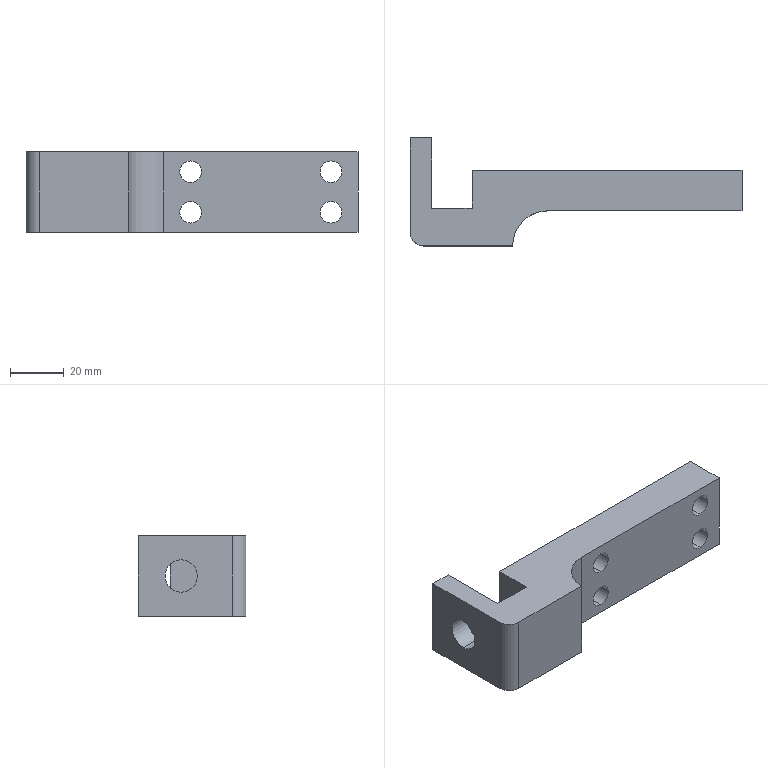Part | SolidWorks | features BaseBody 1 | 1 solid | 23 faces | box 123 x 40 x 30 mm | volume 63756 mm3 | cylinder 12 | plane 11 | commonest cylinder face diameters 8 x8 12 x2 10 x1 26 x1
STEP:
#1=CARTESIAN_POINT('',(340.,-80.,133.121));
#2=VERTEX_POINT('',#1);
#3=CARTESIAN_POINT('',(340.,-80.,141.121));
#4=VERTEX_POINT('',#3);
#5=CARTESIAN_POINT('',(340.,-80.,137.121));
#6=DIRECTION('',(0.,1.,0.));
#7=DIRECTION('',(0.,0.,-1.));
#8=AXIS2_PLACEMENT_3D('',#5,#6,#7);
#9=CIRCLE('',#8,4.);
#10=EDGE_CURVE('',#2,#4,#9,.T.);
#11=ORIENTED_EDGE('',*,*,#10,.T.);
#12=CARTESIAN_POINT('',(340.,-95.,141.121));
#13=VERTEX_POINT('',#12);
#14=CARTESIAN_POINT('',(340.,-95.,141.121));
#15=DIRECTION('',(0.,-1.,0.));
#16=VECTOR('',#15,1000.);
#17=LINE('',#14,#16);
#18=EDGE_CURVE('',#4,#13,#17,.T.);
#19=ORIENTED_EDGE('',*,*,#18,.T.);
#20=CARTESIAN_POINT('',(340.,-95.,133.121));
#21=VERTEX_POINT('',#20);
#22=CARTESIAN_POINT('',(340.,-95.,137.121));
#23=DIRECTION('',(0.,1.,0.));
#24=DIRECTION('',(0.,0.,-1.));
#25=AXIS2_PLACEMENT_3D('',#22,#23,#24);
#26=CIRCLE('',#25,4.);
#27=EDGE_CURVE('',#21,#13,#26,.T.);
#28=ORIENTED_EDGE('',*,*,#27,.F.);
#29=CARTESIAN_POINT('',(340.,-95.,133.121));
#30=DIRECTION('',(0.,-1.,0.));
#31=VECTOR('',#30,1000.);
#32=LINE('',#29,#31);
#33=EDGE_CURVE('',#2,#21,#32,.T.);
#34=ORIENTED_EDGE('',*,*,#33,.F.);
#35=EDGE_LOOP('',(#11,#19,#28,#34));
#36=FACE_OUTER_BOUND('',#35,.T.);
#37=CARTESIAN_POINT('',(340.,-95.,137.121));
#38=DIRECTION('',(0.,-1.,0.));
#39=DIRECTION('',(0.,0.,-1.));
#40=AXIS2_PLACEMENT_3D('',#37,#38,#39);
#41=CYLINDRICAL_SURFACE('',#40,4.);
#42=ADVANCED_FACE('',(#36),#41,.F.);
#43=CARTESIAN_POINT('',(340.,-80.,148.121));
#44=VERTEX_POINT('',#43);
#45=CARTESIAN_POINT('',(340.,-80.,156.121));
#46=VERTEX_POINT('',#45);
#47=CARTESIAN_POINT('',(340.,-80.,152.121));
#48=DIRECTION('',(0.,1.,0.));
#49=DIRECTION('',(0.,0.,-1.));
#50=AXIS2_PLACEMENT_3D('',#47,#48,#49);
#51=CIRCLE('',#50,4.);
#52=EDGE_CURVE('',#44,#46,#51,.T.);
#53=ORIENTED_EDGE('',*,*,#52,.T.);
#54=CARTESIAN_POINT('',(340.,-95.,156.121));
#55=VERTEX_POINT('',#54);
#56=CARTESIAN_POINT('',(340.,-95.,156.121));
#57=DIRECTION('',(0.,-1.,0.));
#58=VECTOR('',#57,1000.);
#59=LINE('',#56,#58);
#60=EDGE_CURVE('',#46,#55,#59,.T.);
#61=ORIENTED_EDGE('',*,*,#60,.T.);
#62=CARTESIAN_POINT('',(340.,-95.,148.121));
#63=VERTEX_POINT('',#62);
#64=CARTESIAN_POINT('',(340.,-95.,152.121));
#65=DIRECTION('',(0.,1.,0.));
#66=DIRECTION('',(0.,0.,-1.));
#67=AXIS2_PLACEMENT_3D('',#64,#65,#66);
#68=CIRCLE('',#67,4.);
#69=EDGE_CURVE('',#63,#55,#68,.T.);
#70=ORIENTED_EDGE('',*,*,#69,.F.);
#71=CARTESIAN_POINT('',(340.,-95.,148.121));
#72=DIRECTION('',(0.,-1.,0.));
#73=VECTOR('',#72,1000.);
#74=LINE('',#71,#73);
#75=EDGE_CURVE('',#44,#63,#74,.T.);
#76=ORIENTED_EDGE('',*,*,#75,.F.);
#77=EDGE_LOOP('',(#53,#61,#70,#76));
#78=FACE_OUTER_BOUND('',#77,.T.);
#79=CARTESIAN_POINT('',(340.,-95.,152.121));
#80=DIRECTION('',(0.,-1.,0.));
#81=DIRECTION('',(0.,0.,-1.));
#82=AXIS2_PLACEMENT_3D('',#79,#80,#81);
#83=CYLINDRICAL_SURFACE('',#82,4.);
#84=ADVANCED_FACE('',(#78),#83,.F.);
#85=CARTESIAN_POINT('',(288.,-80.,148.121));
#86=VERTEX_POINT('',#85);
#87=CARTESIAN_POINT('',(288.,-80.,156.121));
#88=VERTEX_POINT('',#87);
#89=CARTESIAN_POINT('',(288.,-80.,152.121));
#90=DIRECTION('',(0.,1.,0.));
#91=DIRECTION('',(0.,0.,-1.));
#92=AXIS2_PLACEMENT_3D('',#89,#90,#91);
#93=CIRCLE('',#92,4.);
#94=EDGE_CURVE('',#86,#88,#93,.T.);
#95=ORIENTED_EDGE('',*,*,#94,.T.);
#96=CARTESIAN_POINT('',(288.,-95.,156.121));
#97=VERTEX_POINT('',#96);
#98=CARTESIAN_POINT('',(288.,-95.,156.121));
#99=DIRECTION('',(0.,-1.,0.));
#100=VECTOR('',#99,1000.);
#101=LINE('',#98,#100);
#102=EDGE_CURVE('',#88,#97,#101,.T.);
#103=ORIENTED_EDGE('',*,*,#102,.T.);
#104=CARTESIAN_POINT('',(288.,-95.,148.121));
#105=VERTEX_POINT('',#104);
#106=CARTESIAN_POINT('',(288.,-95.,152.121));
#107=DIRECTION('',(0.,1.,0.));
#108=DIRECTION('',(0.,0.,-1.));
#109=AXIS2_PLACEMENT_3D('',#106,#107,#108);
#110=CIRCLE('',#109,4.);
#111=EDGE_CURVE('',#105,#97,#110,.T.);
#112=ORIENTED_EDGE('',*,*,#111,.F.);
#113=CARTESIAN_POINT('',(288.,-95.,148.121));
#114=DIRECTION('',(0.,-1.,0.));
#115=VECTOR('',#114,1000.);
#116=LINE('',#113,#115);
#117=EDGE_CURVE('',#86,#105,#116,.T.);
#118=ORIENTED_EDGE('',*,*,#117,.F.);
#119=EDGE_LOOP('',(#95,#103,#112,#118));
#120=FACE_OUTER_BOUND('',#119,.T.);
#121=CARTESIAN_POINT('',(288.,-95.,152.121));
#122=DIRECTION('',(0.,-1.,0.));
#123=DIRECTION('',(0.,0.,-1.));
#124=AXIS2_PLACEMENT_3D('',#121,#122,#123);
#125=CYLINDRICAL_SURFACE('',#124,4.);
#126=ADVANCED_FACE('',(#120),#125,.F.);
#127=CARTESIAN_POINT('',(288.,-80.,133.121));
#128=VERTEX_POINT('',#127);
#129=CARTESIAN_POINT('',(288.,-80.,141.121));
#130=VERTEX_POINT('',#129);
#131=CARTESIAN_POINT('',(288.,-80.,137.121));
#132=DIRECTION('',(0.,1.,0.));
#133=DIRECTION('',(0.,0.,-1.));
#134=AXIS2_PLACEMENT_3D('',#131,#132,#133);
#135=CIRCLE('',#134,4.);
#136=EDGE_CURVE('',#128,#130,#135,.T.);
#137=ORIENTED_EDGE('',*,*,#136,.T.);
#138=CARTESIAN_POINT('',(288.,-95.,141.121));
#139=VERTEX_POINT('',#138);
#140=CARTESIAN_POINT('',(288.,-95.,141.121));
#141=DIRECTION('',(0.,-1.,0.));
#142=VECTOR('',#141,1000.);
#143=LINE('',#140,#142);
#144=EDGE_CURVE('',#130,#139,#143,.T.);
#145=ORIENTED_EDGE('',*,*,#144,.T.);
#146=CARTESIAN_POINT('',(288.,-95.,133.121));
#147=VERTEX_POINT('',#146);
#148=CARTESIAN_POINT('',(288.,-95.,137.121));
#149=DIRECTION('',(0.,1.,0.));
#150=DIRECTION('',(0.,0.,-1.));
#151=AXIS2_PLACEMENT_3D('',#148,#149,#150);
#152=CIRCLE('',#151,4.);
#153=EDGE_CURVE('',#147,#139,#152,.T.);
#154=ORIENTED_EDGE('',*,*,#153,.F.);
#155=CARTESIAN_POINT('',(288.,-95.,133.121));
#156=DIRECTION('',(0.,-1.,0.));
#157=VECTOR('',#156,1000.);
#158=LINE('',#155,#157);
#159=EDGE_CURVE('',#128,#147,#158,.T.);
#160=ORIENTED_EDGE('',*,*,#159,.F.);
#161=EDGE_LOOP('',(#137,#145,#154,#160));
#162=FACE_OUTER_BOUND('',#161,.T.);
#163=CARTESIAN_POINT('',(288.,-95.,137.121));
#164=DIRECTION('',(0.,-1.,0.));
#165=DIRECTION('',(0.,0.,-1.));
#166=AXIS2_PLACEMENT_3D('',#163,#164,#165);
#167=CYLINDRICAL_SURFACE('',#166,4.);
#168=ADVANCED_FACE('',(#162),#167,.F.);
#169=CARTESIAN_POINT('',(235.,-84.,150.621));
#170=VERTEX_POINT('',#169);
#171=CARTESIAN_POINT('',(235.,-84.,138.621));
#172=VERTEX_POINT('',#171);
#173=CARTESIAN_POINT('',(235.,-84.,144.621));
#174=DIRECTION('',(1.,0.,0.));
#175=DIRECTION('',(0.,0.,1.));
#176=AXIS2_PLACEMENT_3D('',#173,#174,#175);
#177=CIRCLE('',#176,6.);
#178=EDGE_CURVE('',#170,#172,#177,.T.);
#179=ORIENTED_EDGE('',*,*,#178,.T.);
#180=CARTESIAN_POINT('',(227.,-84.,138.621));
#181=VERTEX_POINT('',#180);
#182=CARTESIAN_POINT('',(251.971,-84.,138.621));
#183=DIRECTION('',(-1.,0.,0.));
#184=VECTOR('',#183,1000.);
#185=LINE('',#182,#184);
#186=EDGE_CURVE('',#172,#181,#185,.T.);
#187=ORIENTED_EDGE('',*,*,#186,.T.);
#188=CARTESIAN_POINT('',(227.,-84.,150.621));
#189=VERTEX_POINT('',#188);
#190=CARTESIAN_POINT('',(227.,-84.,144.621));
#191=DIRECTION('',(-1.,0.,0.));
#192=DIRECTION('',(0.,0.,1.));
#193=AXIS2_PLACEMENT_3D('',#190,#191,#192);
#194=CIRCLE('',#193,6.);
#195=EDGE_CURVE('',#181,#189,#194,.T.);
#196=ORIENTED_EDGE('',*,*,#195,.T.);
#197=CARTESIAN_POINT('',(251.971,-84.,150.621));
#198=DIRECTION('',(-1.,0.,0.));
#199=VECTOR('',#198,1000.);
#200=LINE('',#197,#199);
#201=EDGE_CURVE('',#170,#189,#200,.T.);
#202=ORIENTED_EDGE('',*,*,#201,.F.);
#203=EDGE_LOOP('',(#179,#187,#196,#202));
#204=FACE_OUTER_BOUND('',#203,.T.);
#205=CARTESIAN_POINT('',(251.971,-84.,144.621));
#206=DIRECTION('',(-1.,0.,0.));
#207=DIRECTION('',(0.,0.,1.));
#208=AXIS2_PLACEMENT_3D('',#205,#206,#207);
#209=CYLINDRICAL_SURFACE('',#208,6.);
#210=ADVANCED_FACE('',(#204),#209,.F.);
#211=CARTESIAN_POINT('',(350.,-80.,129.621));
#212=VERTEX_POINT('',#211);
#213=CARTESIAN_POINT('',(350.,-80.,159.621));
#214=VERTEX_POINT('',#213);
#215=CARTESIAN_POINT('',(350.,-80.,129.621));
#216=DIRECTION('',(0.,0.,1.));
#217=VECTOR('',#216,1000.);
#218=LINE('',#215,#217);
#219=EDGE_CURVE('',#212,#214,#218,.T.);
#220=ORIENTED_EDGE('',*,*,#219,.F.);
#221=CARTESIAN_POINT('',(250.,-80.,129.621));
#222=VERTEX_POINT('',#221);
#223=CARTESIAN_POINT('',(350.,-80.,129.621));
#224=DIRECTION('',(1.,0.,0.));
#225=VECTOR('',#224,1000.);
#226=LINE('',#223,#225);
#227=EDGE_CURVE('',#222,#212,#226,.T.);
#228=ORIENTED_EDGE('',*,*,#227,.F.);
#229=CARTESIAN_POINT('',(250.,-80.,159.621));
#230=VERTEX_POINT('',#229);
#231=CARTESIAN_POINT('',(250.,-80.,129.621));
#232=DIRECTION('',(0.,0.,-1.));
#233=VECTOR('',#232,1000.);
#234=LINE('',#231,#233);
#235=EDGE_CURVE('',#230,#222,#234,.T.);
#236=ORIENTED_EDGE('',*,*,#235,.F.);
#237=CARTESIAN_POINT('',(350.,-80.,159.621));
#238=DIRECTION('',(-1.,0.,0.));
#239=VECTOR('',#238,1000.);
#240=LINE('',#237,#239);
#241=EDGE_CURVE('',#214,#230,#240,.T.);
#242=ORIENTED_EDGE('',*,*,#241,.F.);
#243=EDGE_LOOP('',(#220,#228,#236,#242));
#244=FACE_OUTER_BOUND('',#243,.T.);
#245=ORIENTED_EDGE('',*,*,#10,.F.);
#246=CARTESIAN_POINT('',(340.,-80.,137.121));
#247=DIRECTION('',(0.,1.,0.));
#248=DIRECTION('',(0.,0.,-1.));
#249=AXIS2_PLACEMENT_3D('',#246,#247,#248);
#250=CIRCLE('',#249,4.);
#251=EDGE_CURVE('',#4,#2,#250,.T.);
#252=ORIENTED_EDGE('',*,*,#251,.F.);
#253=EDGE_LOOP('',(#245,#252));
#254=FACE_BOUND('',#253,.T.);
#255=ORIENTED_EDGE('',*,*,#52,.F.);
#256=CARTESIAN_POINT('',(340.,-80.,152.121));
#257=DIRECTION('',(0.,1.,0.));
#258=DIRECTION('',(0.,0.,-1.));
#259=AXIS2_PLACEMENT_3D('',#256,#257,#258);
#260=CIRCLE('',#259,4.);
#261=EDGE_CURVE('',#46,#44,#260,.T.);
#262=ORIENTED_EDGE('',*,*,#261,.F.);
#263=EDGE_LOOP('',(#255,#262));
#264=FACE_BOUND('',#263,.T.);
#265=ORIENTED_EDGE('',*,*,#94,.F.);
#266=CARTESIAN_POINT('',(288.,-80.,152.121));
#267=DIRECTION('',(0.,1.,0.));
#268=DIRECTION('',(0.,0.,-1.));
#269=AXIS2_PLACEMENT_3D('',#266,#267,#268);
#270=CIRCLE('',#269,4.);
#271=EDGE_CURVE('',#88,#86,#270,.T.);
#272=ORIENTED_EDGE('',*,*,#271,.F.);
#273=EDGE_LOOP('',(#265,#272));
#274=FACE_BOUND('',#273,.T.);
#275=ORIENTED_EDGE('',*,*,#136,.F.);
#276=CARTESIAN_POINT('',(288.,-80.,137.121));
#277=DIRECTION('',(0.,1.,0.));
#278=DIRECTION('',(0.,0.,-1.));
#279=AXIS2_PLACEMENT_3D('',#276,#277,#278);
#280=CIRCLE('',#279,4.);
#281=EDGE_CURVE('',#130,#128,#280,.T.);
#282=ORIENTED_EDGE('',*,*,#281,.F.);
#283=EDGE_LOOP('',(#275,#282));
#284=FACE_BOUND('',#283,.T.);
#285=CARTESIAN_POINT('',(350.,-80.,129.621));
#286=DIRECTION('',(0.,-1.,0.));
#287=DIRECTION('',(0.,0.,-1.));
#288=AXIS2_PLACEMENT_3D('',#285,#286,#287);
#289=PLANE('',#288);
#290=ADVANCED_FACE('',(#244,#254,#264,#274,#284),#289,.F.);
#291=CARTESIAN_POINT('',(232.,-108.,159.621));
#292=VERTEX_POINT('',#291);
#293=CARTESIAN_POINT('',(227.,-103.,159.621));
#294=VERTEX_POINT('',#293);
#295=CARTESIAN_POINT('',(232.,-103.,159.621));
#296=DIRECTION('',(0.,0.,-1.));
#297=DIRECTION('',(1.,0.,0.));
#298=AXIS2_PLACEMENT_3D('',#295,#296,#297);
#299=CIRCLE('',#298,5.);
#300=EDGE_CURVE('',#292,#294,#299,.T.);
#301=ORIENTED_EDGE('',*,*,#300,.F.);
#302=CARTESIAN_POINT('',(265.,-108.,159.621));
#303=VERTEX_POINT('',#302);
#304=CARTESIAN_POINT('',(251.867,-108.,159.621));
#305=DIRECTION('',(-1.,0.,0.));
#306=VECTOR('',#305,1000.);
#307=LINE('',#304,#306);
#308=EDGE_CURVE('',#303,#292,#307,.T.);
#309=ORIENTED_EDGE('',*,*,#308,.F.);
#310=CARTESIAN_POINT('',(278.,-95.,159.621));
#311=VERTEX_POINT('',#310);
#312=CARTESIAN_POINT('',(278.,-108.,159.621));
#313=DIRECTION('',(0.,0.,1.));
#314=DIRECTION('',(-1.,0.,0.));
#315=AXIS2_PLACEMENT_3D('',#312,#313,#314);
#316=CIRCLE('',#315,13.);
#317=EDGE_CURVE('',#311,#303,#316,.T.);
#318=ORIENTED_EDGE('',*,*,#317,.F.);
#319=CARTESIAN_POINT('',(350.,-95.,159.621));
#320=VERTEX_POINT('',#319);
#321=CARTESIAN_POINT('',(251.867,-95.,159.621));
#322=DIRECTION('',(-1.,0.,0.));
#323=VECTOR('',#322,1000.);
#324=LINE('',#321,#323);
#325=EDGE_CURVE('',#320,#311,#324,.T.);
#326=ORIENTED_EDGE('',*,*,#325,.F.);
#327=CARTESIAN_POINT('',(350.,-82.6,159.621));
#328=DIRECTION('',(0.,-1.,0.));
#329=VECTOR('',#328,1000.);
#330=LINE('',#327,#329);
#331=EDGE_CURVE('',#214,#320,#330,.T.);
#332=ORIENTED_EDGE('',*,*,#331,.F.);
#333=ORIENTED_EDGE('',*,*,#241,.T.);
#334=CARTESIAN_POINT('',(250.,-94.,159.621));
#335=VERTEX_POINT('',#334);
#336=CARTESIAN_POINT('',(250.,-82.6,159.621));
#337=DIRECTION('',(0.,1.,0.));
#338=VECTOR('',#337,1000.);
#339=LINE('',#336,#338);
#340=EDGE_CURVE('',#335,#230,#339,.T.);
#341=ORIENTED_EDGE('',*,*,#340,.F.);
#342=CARTESIAN_POINT('',(235.,-94.,159.621));
#343=VERTEX_POINT('',#342);
#344=CARTESIAN_POINT('',(251.867,-94.,159.621));
#345=DIRECTION('',(1.,0.,0.));
#346=VECTOR('',#345,1000.);
#347=LINE('',#344,#346);
#348=EDGE_CURVE('',#343,#335,#347,.T.);
#349=ORIENTED_EDGE('',*,*,#348,.F.);
#350=CARTESIAN_POINT('',(235.,-68.,159.621));
#351=VERTEX_POINT('',#350);
#352=CARTESIAN_POINT('',(235.,-82.6,159.621));
#353=DIRECTION('',(0.,-1.,0.));
#354=VECTOR('',#353,1000.);
#355=LINE('',#352,#354);
#356=EDGE_CURVE('',#351,#343,#355,.T.);
#357=ORIENTED_EDGE('',*,*,#356,.F.);
#358=CARTESIAN_POINT('',(227.,-68.,159.621));
#359=VERTEX_POINT('',#358);
#360=CARTESIAN_POINT('',(251.867,-68.,159.621));
#361=DIRECTION('',(1.,0.,0.));
#362=VECTOR('',#361,1000.);
#363=LINE('',#360,#362);
#364=EDGE_CURVE('',#359,#351,#363,.T.);
#365=ORIENTED_EDGE('',*,*,#364,.F.);
#366=CARTESIAN_POINT('',(227.,-82.6,159.621));
#367=DIRECTION('',(0.,1.,0.));
#368=VECTOR('',#367,1000.);
#369=LINE('',#366,#368);
#370=EDGE_CURVE('',#294,#359,#369,.T.);
#371=ORIENTED_EDGE('',*,*,#370,.F.);
#372=EDGE_LOOP('',(#301,#309,#318,#326,#332,#333,#341,#349,#357,#365,#371));
#373=FACE_OUTER_BOUND('',#372,.T.);
#374=CARTESIAN_POINT('',(251.867,-82.6,159.621));
#375=DIRECTION('',(0.,0.,-1.));
#376=DIRECTION('',(-1.,0.,0.));
#377=AXIS2_PLACEMENT_3D('',#374,#375,#376);
#378=PLANE('',#377);
#379=ADVANCED_FACE('',(#373),#378,.F.);
#380=CARTESIAN_POINT('',(350.,-95.,129.621));
#381=VERTEX_POINT('',#380);
#382=CARTESIAN_POINT('',(350.,-95.,129.621));
#383=DIRECTION('',(0.,0.,1.));
#384=VECTOR('',#383,1000.);
#385=LINE('',#382,#384);
#386=EDGE_CURVE('',#381,#320,#385,.T.);
#387=ORIENTED_EDGE('',*,*,#386,.F.);
#388=CARTESIAN_POINT('',(350.,-80.,129.621));
#389=DIRECTION('',(0.,-1.,0.));
#390=VECTOR('',#389,1000.);
#391=LINE('',#388,#390);
#392=EDGE_CURVE('',#212,#381,#391,.T.);
#393=ORIENTED_EDGE('',*,*,#392,.F.);
#394=ORIENTED_EDGE('',*,*,#219,.T.);
#395=ORIENTED_EDGE('',*,*,#331,.T.);
#396=EDGE_LOOP('',(#387,#393,#394,#395));
#397=FACE_OUTER_BOUND('',#396,.T.);
#398=CARTESIAN_POINT('',(350.,-80.,129.621));
#399=DIRECTION('',(-1.,0.,0.));
#400=DIRECTION('',(0.,0.,1.));
#401=AXIS2_PLACEMENT_3D('',#398,#399,#400);
#402=PLANE('',#401);
#403=ADVANCED_FACE('',(#397),#402,.F.);
#404=CARTESIAN_POINT('',(278.,-95.,129.621));
#405=VERTEX_POINT('',#404);
#406=CARTESIAN_POINT('',(251.867,-95.,129.621));
#407=DIRECTION('',(-1.,0.,0.));
#408=VECTOR('',#407,1000.);
#409=LINE('',#406,#408);
#410=EDGE_CURVE('',#381,#405,#409,.T.);
#411=ORIENTED_EDGE('',*,*,#410,.T.);
#412=CARTESIAN_POINT('',(265.,-108.,129.621));
#413=VERTEX_POINT('',#412);
#414=CARTESIAN_POINT('',(278.,-108.,129.621));
#415=DIRECTION('',(0.,0.,1.));
#416=DIRECTION('',(-1.,0.,0.));
#417=AXIS2_PLACEMENT_3D('',#414,#415,#416);
#418=CIRCLE('',#417,13.);
#419=EDGE_CURVE('',#405,#413,#418,.T.);
#420=ORIENTED_EDGE('',*,*,#419,.T.);
#421=CARTESIAN_POINT('',(232.,-108.,129.621));
#422=VERTEX_POINT('',#421);
#423=CARTESIAN_POINT('',(251.867,-108.,129.621));
#424=DIRECTION('',(-1.,0.,0.));
#425=VECTOR('',#424,1000.);
#426=LINE('',#423,#425);
#427=EDGE_CURVE('',#413,#422,#426,.T.);
#428=ORIENTED_EDGE('',*,*,#427,.T.);
#429=CARTESIAN_POINT('',(227.,-103.,129.621));
#430=VERTEX_POINT('',#429);
#431=CARTESIAN_POINT('',(232.,-103.,129.621));
#432=DIRECTION('',(0.,0.,-1.));
#433=DIRECTION('',(1.,0.,0.));
#434=AXIS2_PLACEMENT_3D('',#431,#432,#433);
#435=CIRCLE('',#434,5.);
#436=EDGE_CURVE('',#422,#430,#435,.T.);
#437=ORIENTED_EDGE('',*,*,#436,.T.);
#438=CARTESIAN_POINT('',(227.,-68.,129.621));
#439=VERTEX_POINT('',#438);
#440=CARTESIAN_POINT('',(227.,-82.6,129.621));
#441=DIRECTION('',(0.,1.,0.));
#442=VECTOR('',#441,1000.);
#443=LINE('',#440,#442);
#444=EDGE_CURVE('',#430,#439,#443,.T.);
#445=ORIENTED_EDGE('',*,*,#444,.T.);
#446=CARTESIAN_POINT('',(235.,-68.,129.621));
#447=VERTEX_POINT('',#446);
#448=CARTESIAN_POINT('',(251.867,-68.,129.621));
#449=DIRECTION('',(1.,0.,0.));
#450=VECTOR('',#449,1000.);
#451=LINE('',#448,#450);
#452=EDGE_CURVE('',#439,#447,#451,.T.);
#453=ORIENTED_EDGE('',*,*,#452,.T.);
#454=CARTESIAN_POINT('',(235.,-94.,129.621));
#455=VERTEX_POINT('',#454);
#456=CARTESIAN_POINT('',(235.,-82.6,129.621));
#457=DIRECTION('',(0.,-1.,0.));
#458=VECTOR('',#457,1000.);
#459=LINE('',#456,#458);
#460=EDGE_CURVE('',#447,#455,#459,.T.);
#461=ORIENTED_EDGE('',*,*,#460,.T.);
#462=CARTESIAN_POINT('',(250.,-94.,129.621));
#463=VERTEX_POINT('',#462);
#464=CARTESIAN_POINT('',(251.867,-94.,129.621));
#465=DIRECTION('',(1.,0.,0.));
#466=VECTOR('',#465,1000.);
#467=LINE('',#464,#466);
#468=EDGE_CURVE('',#455,#463,#467,.T.);
#469=ORIENTED_EDGE('',*,*,#468,.T.);
#470=CARTESIAN_POINT('',(250.,-82.6,129.621));
#471=DIRECTION('',(0.,1.,0.));
#472=VECTOR('',#471,1000.);
#473=LINE('',#470,#472);
#474=EDGE_CURVE('',#463,#222,#473,.T.);
#475=ORIENTED_EDGE('',*,*,#474,.T.);
#476=ORIENTED_EDGE('',*,*,#227,.T.);
#477=ORIENTED_EDGE('',*,*,#392,.T.);
#478=EDGE_LOOP('',(#411,#420,#428,#437,#445,#453,#461,#469,#475,#476,#477));
#479=FACE_OUTER_BOUND('',#478,.T.);
#480=CARTESIAN_POINT('',(251.867,-82.6,129.621));
#481=DIRECTION('',(0.,0.,-1.));
#482=DIRECTION('',(-1.,0.,0.));
#483=AXIS2_PLACEMENT_3D('',#480,#481,#482);
#484=PLANE('',#483);
#485=ADVANCED_FACE('',(#479),#484,.T.);
#486=ORIENTED_EDGE('',*,*,#235,.T.);
#487=ORIENTED_EDGE('',*,*,#474,.F.);
#488=CARTESIAN_POINT('',(250.,-94.,129.621));
#489=DIRECTION('',(0.,0.,-1.));
#490=VECTOR('',#489,1000.);
#491=LINE('',#488,#490);
#492=EDGE_CURVE('',#335,#463,#491,.T.);
#493=ORIENTED_EDGE('',*,*,#492,.F.);
#494=ORIENTED_EDGE('',*,*,#340,.T.);
#495=EDGE_LOOP('',(#486,#487,#493,#494));
#496=FACE_OUTER_BOUND('',#495,.T.);
#497=CARTESIAN_POINT('',(250.,-80.,129.621));
#498=DIRECTION('',(1.,0.,0.));
#499=DIRECTION('',(0.,0.,-1.));
#500=AXIS2_PLACEMENT_3D('',#497,#498,#499);
#501=PLANE('',#500);
#502=ADVANCED_FACE('',(#496),#501,.F.);
#503=ORIENTED_EDGE('',*,*,#18,.F.);
#504=ORIENTED_EDGE('',*,*,#251,.T.);
#505=ORIENTED_EDGE('',*,*,#33,.T.);
#506=CARTESIAN_POINT('',(340.,-95.,137.121));
#507=DIRECTION('',(0.,1.,0.));
#508=DIRECTION('',(0.,0.,-1.));
#509=AXIS2_PLACEMENT_3D('',#506,#507,#508);
#510=CIRCLE('',#509,4.);
#511=EDGE_CURVE('',#13,#21,#510,.T.);
#512=ORIENTED_EDGE('',*,*,#511,.F.);
#513=EDGE_LOOP('',(#503,#504,#505,#512));
#514=FACE_OUTER_BOUND('',#513,.T.);
#515=CARTESIAN_POINT('',(340.,-95.,137.121));
#516=DIRECTION('',(0.,-1.,0.));
#517=DIRECTION('',(0.,0.,-1.));
#518=AXIS2_PLACEMENT_3D('',#515,#516,#517);
#519=CYLINDRICAL_SURFACE('',#518,4.);
#520=ADVANCED_FACE('',(#514),#519,.F.);
#521=ORIENTED_EDGE('',*,*,#60,.F.);
#522=ORIENTED_EDGE('',*,*,#261,.T.);
#523=ORIENTED_EDGE('',*,*,#75,.T.);
#524=CARTESIAN_POINT('',(340.,-95.,152.121));
#525=DIRECTION('',(0.,1.,0.));
#526=DIRECTION('',(0.,0.,-1.));
#527=AXIS2_PLACEMENT_3D('',#524,#525,#526);
#528=CIRCLE('',#527,4.);
#529=EDGE_CURVE('',#55,#63,#528,.T.);
#530=ORIENTED_EDGE('',*,*,#529,.F.);
#531=EDGE_LOOP('',(#521,#522,#523,#530));
#532=FACE_OUTER_BOUND('',#531,.T.);
#533=CARTESIAN_POINT('',(340.,-95.,152.121));
#534=DIRECTION('',(0.,-1.,0.));
#535=DIRECTION('',(0.,0.,-1.));
#536=AXIS2_PLACEMENT_3D('',#533,#534,#535);
#537=CYLINDRICAL_SURFACE('',#536,4.);
#538=ADVANCED_FACE('',(#532),#537,.F.);
#539=ORIENTED_EDGE('',*,*,#102,.F.);
#540=ORIENTED_EDGE('',*,*,#271,.T.);
#541=ORIENTED_EDGE('',*,*,#117,.T.);
#542=CARTESIAN_POINT('',(288.,-95.,152.121));
#543=DIRECTION('',(0.,1.,0.));
#544=DIRECTION('',(0.,0.,-1.));
#545=AXIS2_PLACEMENT_3D('',#542,#543,#544);
#546=CIRCLE('',#545,4.);
#547=EDGE_CURVE('',#97,#105,#546,.T.);
#548=ORIENTED_EDGE('',*,*,#547,.F.);
#549=EDGE_LOOP('',(#539,#540,#541,#548));
#550=FACE_OUTER_BOUND('',#549,.T.);
#551=CARTESIAN_POINT('',(288.,-95.,152.121));
#552=DIRECTION('',(0.,-1.,0.));
#553=DIRECTION('',(0.,0.,-1.));
#554=AXIS2_PLACEMENT_3D('',#551,#552,#553);
#555=CYLINDRICAL_SURFACE('',#554,4.);
#556=ADVANCED_FACE('',(#550),#555,.F.);
#557=ORIENTED_EDGE('',*,*,#144,.F.);
#558=ORIENTED_EDGE('',*,*,#281,.T.);
#559=ORIENTED_EDGE('',*,*,#159,.T.);
#560=CARTESIAN_POINT('',(288.,-95.,137.121));
#561=DIRECTION('',(0.,1.,0.));
#562=DIRECTION('',(0.,0.,-1.));
#563=AXIS2_PLACEMENT_3D('',#560,#561,#562);
#564=CIRCLE('',#563,4.);
#565=EDGE_CURVE('',#139,#147,#564,.T.);
#566=ORIENTED_EDGE('',*,*,#565,.F.);
#567=EDGE_LOOP('',(#557,#558,#559,#566));
#568=FACE_OUTER_BOUND('',#567,.T.);
#569=CARTESIAN_POINT('',(288.,-95.,137.121));
#570=DIRECTION('',(0.,-1.,0.));
#571=DIRECTION('',(0.,0.,-1.));
#572=AXIS2_PLACEMENT_3D('',#569,#570,#571);
#573=CYLINDRICAL_SURFACE('',#572,4.);
#574=ADVANCED_FACE('',(#568),#573,.F.);
#575=CARTESIAN_POINT('',(227.,-103.,129.621));
#576=DIRECTION('',(0.,0.,-1.));
#577=VECTOR('',#576,1000.);
#578=LINE('',#575,#577);
#579=EDGE_CURVE('',#294,#430,#578,.T.);
#580=ORIENTED_EDGE('',*,*,#579,.F.);
#581=ORIENTED_EDGE('',*,*,#370,.T.);
#582=CARTESIAN_POINT('',(227.,-68.,129.621));
#583=DIRECTION('',(0.,0.,1.));
#584=VECTOR('',#583,1000.);
#585=LINE('',#582,#584);
#586=EDGE_CURVE('',#439,#359,#585,.T.);
#587=ORIENTED_EDGE('',*,*,#586,.F.);
#588=ORIENTED_EDGE('',*,*,#444,.F.);
#589=EDGE_LOOP('',(#580,#581,#587,#588));
#590=FACE_OUTER_BOUND('',#589,.T.);
#591=CARTESIAN_POINT('',(227.,-84.,144.621));
#592=DIRECTION('',(-1.,0.,0.));
#593=DIRECTION('',(0.,0.,1.));
#594=AXIS2_PLACEMENT_3D('',#591,#592,#593);
#595=CIRCLE('',#594,6.);
#596=EDGE_CURVE('',#189,#181,#595,.T.);
#597=ORIENTED_EDGE('',*,*,#596,.F.);
#598=ORIENTED_EDGE('',*,*,#195,.F.);
#599=EDGE_LOOP('',(#597,#598));
#600=FACE_BOUND('',#599,.T.);
#601=CARTESIAN_POINT('',(227.,-93.,129.621));
#602=DIRECTION('',(1.,0.,0.));
#603=DIRECTION('',(0.,0.,-1.));
#604=AXIS2_PLACEMENT_3D('',#601,#602,#603);
#605=PLANE('',#604);
#606=ADVANCED_FACE('',(#590,#600),#605,.F.);
#607=ORIENTED_EDGE('',*,*,#300,.T.);
#608=ORIENTED_EDGE('',*,*,#579,.T.);
#609=ORIENTED_EDGE('',*,*,#436,.F.);
#610=CARTESIAN_POINT('',(232.,-108.,129.621));
#611=DIRECTION('',(0.,0.,1.));
#612=VECTOR('',#611,1000.);
#613=LINE('',#610,#612);
#614=EDGE_CURVE('',#422,#292,#613,.T.);
#615=ORIENTED_EDGE('',*,*,#614,.T.);
#616=EDGE_LOOP('',(#607,#608,#609,#615));
#617=FACE_OUTER_BOUND('',#616,.T.);
#618=CARTESIAN_POINT('',(232.,-103.,129.621));
#619=DIRECTION('',(0.,0.,1.));
#620=DIRECTION('',(1.,0.,0.));
#621=AXIS2_PLACEMENT_3D('',#618,#619,#620);
#622=CYLINDRICAL_SURFACE('',#621,5.);
#623=ADVANCED_FACE('',(#617),#622,.T.);
#624=ORIENTED_EDGE('',*,*,#614,.F.);
#625=ORIENTED_EDGE('',*,*,#427,.F.);
#626=CARTESIAN_POINT('',(265.,-108.,129.621));
#627=DIRECTION('',(0.,0.,-1.));
#628=VECTOR('',#627,1000.);
#629=LINE('',#626,#628);
#630=EDGE_CURVE('',#303,#413,#629,.T.);
#631=ORIENTED_EDGE('',*,*,#630,.F.);
#632=ORIENTED_EDGE('',*,*,#308,.T.);
#633=EDGE_LOOP('',(#624,#625,#631,#632));
#634=FACE_OUTER_BOUND('',#633,.T.);
#635=CARTESIAN_POINT('',(265.,-108.,129.621));
#636=DIRECTION('',(0.,1.,0.));
#637=DIRECTION('',(0.,0.,1.));
#638=AXIS2_PLACEMENT_3D('',#635,#636,#637);
#639=PLANE('',#638);
#640=ADVANCED_FACE('',(#634),#639,.F.);
#641=CARTESIAN_POINT('',(278.,-95.,129.621));
#642=DIRECTION('',(0.,0.,-1.));
#643=VECTOR('',#642,1000.);
#644=LINE('',#641,#643);
#645=EDGE_CURVE('',#311,#405,#644,.T.);
#646=ORIENTED_EDGE('',*,*,#645,.F.);
#647=ORIENTED_EDGE('',*,*,#317,.T.);
#648=ORIENTED_EDGE('',*,*,#630,.T.);
#649=ORIENTED_EDGE('',*,*,#419,.F.);
#650=EDGE_LOOP('',(#646,#647,#648,#649));
#651=FACE_OUTER_BOUND('',#650,.T.);
#652=CARTESIAN_POINT('',(278.,-108.,129.621));
#653=DIRECTION('',(0.,0.,-1.));
#654=DIRECTION('',(-1.,0.,0.));
#655=AXIS2_PLACEMENT_3D('',#652,#653,#654);
#656=CYLINDRICAL_SURFACE('',#655,13.);
#657=ADVANCED_FACE('',(#651),#656,.F.);
#658=ORIENTED_EDGE('',*,*,#645,.T.);
#659=ORIENTED_EDGE('',*,*,#410,.F.);
#660=ORIENTED_EDGE('',*,*,#386,.T.);
#661=ORIENTED_EDGE('',*,*,#325,.T.);
#662=EDGE_LOOP('',(#658,#659,#660,#661));
#663=FACE_OUTER_BOUND('',#662,.T.);
#664=ORIENTED_EDGE('',*,*,#27,.T.);
#665=ORIENTED_EDGE('',*,*,#511,.T.);
#666=EDGE_LOOP('',(#664,#665));
#667=FACE_BOUND('',#666,.T.);
#668=ORIENTED_EDGE('',*,*,#69,.T.);
#669=ORIENTED_EDGE('',*,*,#529,.T.);
#670=EDGE_LOOP('',(#668,#669));
#671=FACE_BOUND('',#670,.T.);
#672=ORIENTED_EDGE('',*,*,#111,.T.);
#673=ORIENTED_EDGE('',*,*,#547,.T.);
#674=EDGE_LOOP('',(#672,#673));
#675=FACE_BOUND('',#674,.T.);
#676=ORIENTED_EDGE('',*,*,#153,.T.);
#677=ORIENTED_EDGE('',*,*,#565,.T.);
#678=EDGE_LOOP('',(#676,#677));
#679=FACE_BOUND('',#678,.T.);
#680=CARTESIAN_POINT('',(350.,-95.,129.621));
#681=DIRECTION('',(0.,1.,0.));
#682=DIRECTION('',(0.,0.,1.));
#683=AXIS2_PLACEMENT_3D('',#680,#681,#682);
#684=PLANE('',#683);
#685=ADVANCED_FACE('',(#663,#667,#671,#675,#679),#684,.F.);
#686=ORIENTED_EDGE('',*,*,#492,.T.);
#687=ORIENTED_EDGE('',*,*,#468,.F.);
#688=CARTESIAN_POINT('',(235.,-94.,129.621));
#689=DIRECTION('',(0.,0.,-1.));
#690=VECTOR('',#689,1000.);
#691=LINE('',#688,#690);
#692=EDGE_CURVE('',#343,#455,#691,.T.);
#693=ORIENTED_EDGE('',*,*,#692,.F.);
#694=ORIENTED_EDGE('',*,*,#348,.T.);
#695=EDGE_LOOP('',(#686,#687,#693,#694));
#696=FACE_OUTER_BOUND('',#695,.T.);
#697=CARTESIAN_POINT('',(250.,-94.,129.621));
#698=DIRECTION('',(0.,-1.,0.));
#699=DIRECTION('',(0.,0.,-1.));
#700=AXIS2_PLACEMENT_3D('',#697,#698,#699);
#701=PLANE('',#700);
#702=ADVANCED_FACE('',(#696),#701,.F.);
#703=ORIENTED_EDGE('',*,*,#692,.T.);
#704=ORIENTED_EDGE('',*,*,#460,.F.);
#705=CARTESIAN_POINT('',(235.,-68.,129.621));
#706=DIRECTION('',(0.,0.,-1.));
#707=VECTOR('',#706,1000.);
#708=LINE('',#705,#707);
#709=EDGE_CURVE('',#351,#447,#708,.T.);
#710=ORIENTED_EDGE('',*,*,#709,.F.);
#711=ORIENTED_EDGE('',*,*,#356,.T.);
#712=EDGE_LOOP('',(#703,#704,#710,#711));
#713=FACE_OUTER_BOUND('',#712,.T.);
#714=ORIENTED_EDGE('',*,*,#178,.F.);
#715=CARTESIAN_POINT('',(235.,-84.,144.621));
#716=DIRECTION('',(1.,0.,0.));
#717=DIRECTION('',(0.,0.,1.));
#718=AXIS2_PLACEMENT_3D('',#715,#716,#717);
#719=CIRCLE('',#718,6.);
#720=EDGE_CURVE('',#172,#170,#719,.T.);
#721=ORIENTED_EDGE('',*,*,#720,.F.);
#722=EDGE_LOOP('',(#714,#721));
#723=FACE_BOUND('',#722,.T.);
#724=CARTESIAN_POINT('',(235.,-94.,129.621));
#725=DIRECTION('',(-1.,0.,0.));
#726=DIRECTION('',(0.,0.,1.));
#727=AXIS2_PLACEMENT_3D('',#724,#725,#726);
#728=PLANE('',#727);
#729=ADVANCED_FACE('',(#713,#723),#728,.F.);
#730=ORIENTED_EDGE('',*,*,#709,.T.);
#731=ORIENTED_EDGE('',*,*,#452,.F.);
#732=ORIENTED_EDGE('',*,*,#586,.T.);
#733=ORIENTED_EDGE('',*,*,#364,.T.);
#734=EDGE_LOOP('',(#730,#731,#732,#733));
#735=FACE_OUTER_BOUND('',#734,.T.);
#736=CARTESIAN_POINT('',(227.,-68.,129.621));
#737=DIRECTION('',(0.,-1.,0.));
#738=DIRECTION('',(0.,0.,-1.));
#739=AXIS2_PLACEMENT_3D('',#736,#737,#738);
#740=PLANE('',#739);
#741=ADVANCED_FACE('',(#735),#740,.F.);
#742=ORIENTED_EDGE('',*,*,#186,.F.);
#743=ORIENTED_EDGE('',*,*,#720,.T.);
#744=ORIENTED_EDGE('',*,*,#201,.T.);
#745=ORIENTED_EDGE('',*,*,#596,.T.);
#746=EDGE_LOOP('',(#742,#743,#744,#745));
#747=FACE_OUTER_BOUND('',#746,.T.);
#748=CARTESIAN_POINT('',(251.971,-84.,144.621));
#749=DIRECTION('',(-1.,0.,0.));
#750=DIRECTION('',(0.,0.,1.));
#751=AXIS2_PLACEMENT_3D('',#748,#749,#750);
#752=CYLINDRICAL_SURFACE('',#751,6.);
#753=ADVANCED_FACE('',(#747),#752,.F.);
#754=CLOSED_SHELL('',(#42,#84,#126,#168,#210,#290,#379,#403,#485,#502,#520,#538,#556,#574,#606,#623,#640,#657,#685,#702,#729,#741,#753));
#755=MANIFOLD_SOLID_BREP('',#754);
#756=CARTESIAN_POINT('',(0.,0.,0.));
#757=DIRECTION('',(0.,0.,1.));
#758=DIRECTION('',(1.,0.,0.));
#759=AXIS2_PLACEMENT_3D('',#756,#757,#758);
#760=(LENGTH_UNIT()NAMED_UNIT(*)SI_UNIT(.MILLI.,.METRE.));
#761=UNCERTAINTY_MEASURE_WITH_UNIT(LENGTH_MEASURE(0.00001),#760,'','');
#762=(NAMED_UNIT(*)PLANE_ANGLE_UNIT()SI_UNIT($,.RADIAN.));
#763=(NAMED_UNIT(*)SI_UNIT($,.STERADIAN.)SOLID_ANGLE_UNIT());
#764=(GEOMETRIC_REPRESENTATION_CONTEXT(3)GLOBAL_UNCERTAINTY_ASSIGNED_CONTEXT((#761))GLOBAL_UNIT_ASSIGNED_CONTEXT((#760,#762,#763))REPRESENTATION_CONTEXT('',''));
#765=ADVANCED_BREP_SHAPE_REPRESENTATION('',(#755,#759),#764);